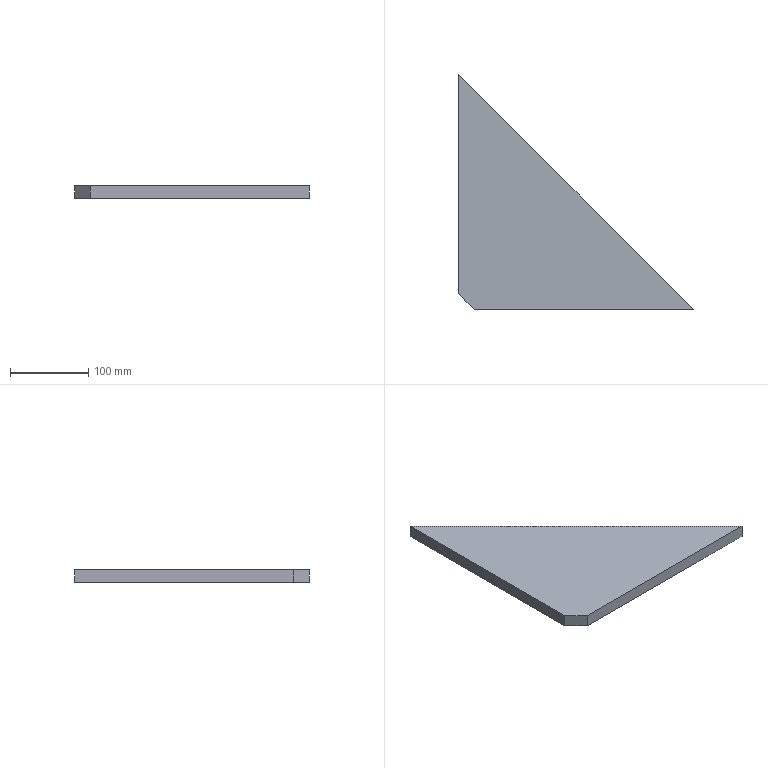Part | SolidWorks | features Chamfer 1, Extrusion 1 | 1 solid | 6 faces | box 300 x 300 x 16 mm | volume 716800 mm3 | plane 6
STEP:
#1=CARTESIAN_POINT('',(0.,20.,-8.));
#2=VERTEX_POINT('',#1);
#3=CARTESIAN_POINT('',(0.,300.,-8.));
#4=VERTEX_POINT('',#3);
#5=CARTESIAN_POINT('',(0.,0.,-8.));
#6=DIRECTION('',(0.,1.,0.));
#7=VECTOR('',#6,1000.);
#8=LINE('',#5,#7);
#9=EDGE_CURVE('',#2,#4,#8,.T.);
#10=ORIENTED_EDGE('',*,*,#9,.F.);
#11=CARTESIAN_POINT('',(0.,20.,8.));
#12=VERTEX_POINT('',#11);
#13=CARTESIAN_POINT('',(0.,20.,8.));
#14=DIRECTION('',(0.,0.,1.));
#15=VECTOR('',#14,1000.);
#16=LINE('',#13,#15);
#17=EDGE_CURVE('',#2,#12,#16,.T.);
#18=ORIENTED_EDGE('',*,*,#17,.T.);
#19=CARTESIAN_POINT('',(0.,300.,8.));
#20=VERTEX_POINT('',#19);
#21=CARTESIAN_POINT('',(0.,0.,8.));
#22=DIRECTION('',(0.,1.,0.));
#23=VECTOR('',#22,1000.);
#24=LINE('',#21,#23);
#25=EDGE_CURVE('',#12,#20,#24,.T.);
#26=ORIENTED_EDGE('',*,*,#25,.T.);
#27=CARTESIAN_POINT('',(0.,300.,8.));
#28=DIRECTION('',(0.,0.,-1.));
#29=VECTOR('',#28,1000.);
#30=LINE('',#27,#29);
#31=EDGE_CURVE('',#20,#4,#30,.T.);
#32=ORIENTED_EDGE('',*,*,#31,.T.);
#33=EDGE_LOOP('',(#10,#18,#26,#32));
#34=FACE_OUTER_BOUND('',#33,.T.);
#35=CARTESIAN_POINT('',(0.,0.,8.));
#36=DIRECTION('',(-1.,0.,0.));
#37=DIRECTION('',(0.,0.,1.));
#38=AXIS2_PLACEMENT_3D('',#35,#36,#37);
#39=PLANE('',#38);
#40=ADVANCED_FACE('',(#34),#39,.T.);
#41=CARTESIAN_POINT('',(300.,0.,8.));
#42=VERTEX_POINT('',#41);
#43=CARTESIAN_POINT('',(20.,0.,8.));
#44=VERTEX_POINT('',#43);
#45=CARTESIAN_POINT('',(300.,0.,8.));
#46=DIRECTION('',(-1.,0.,0.));
#47=VECTOR('',#46,1000.);
#48=LINE('',#45,#47);
#49=EDGE_CURVE('',#42,#44,#48,.T.);
#50=ORIENTED_EDGE('',*,*,#49,.T.);
#51=CARTESIAN_POINT('',(20.,0.,-8.));
#52=VERTEX_POINT('',#51);
#53=CARTESIAN_POINT('',(20.,0.,8.));
#54=DIRECTION('',(0.,0.,-1.));
#55=VECTOR('',#54,1000.);
#56=LINE('',#53,#55);
#57=EDGE_CURVE('',#44,#52,#56,.T.);
#58=ORIENTED_EDGE('',*,*,#57,.T.);
#59=CARTESIAN_POINT('',(300.,0.,-8.));
#60=VERTEX_POINT('',#59);
#61=CARTESIAN_POINT('',(300.,0.,-8.));
#62=DIRECTION('',(-1.,0.,0.));
#63=VECTOR('',#62,1000.);
#64=LINE('',#61,#63);
#65=EDGE_CURVE('',#60,#52,#64,.T.);
#66=ORIENTED_EDGE('',*,*,#65,.F.);
#67=CARTESIAN_POINT('',(300.,0.,8.));
#68=DIRECTION('',(0.,0.,-1.));
#69=VECTOR('',#68,1000.);
#70=LINE('',#67,#69);
#71=EDGE_CURVE('',#42,#60,#70,.T.);
#72=ORIENTED_EDGE('',*,*,#71,.F.);
#73=EDGE_LOOP('',(#50,#58,#66,#72));
#74=FACE_OUTER_BOUND('',#73,.T.);
#75=CARTESIAN_POINT('',(300.,0.,8.));
#76=DIRECTION('',(0.,-1.,0.));
#77=DIRECTION('',(0.,0.,-1.));
#78=AXIS2_PLACEMENT_3D('',#75,#76,#77);
#79=PLANE('',#78);
#80=ADVANCED_FACE('',(#74),#79,.T.);
#81=CARTESIAN_POINT('',(0.,300.,-8.));
#82=DIRECTION('',(0.7071,-0.7071,0.));
#83=VECTOR('',#82,1000.);
#84=LINE('',#81,#83);
#85=EDGE_CURVE('',#4,#60,#84,.T.);
#86=ORIENTED_EDGE('',*,*,#85,.F.);
#87=ORIENTED_EDGE('',*,*,#31,.F.);
#88=CARTESIAN_POINT('',(0.,300.,8.));
#89=DIRECTION('',(0.7071,-0.7071,0.));
#90=VECTOR('',#89,1000.);
#91=LINE('',#88,#90);
#92=EDGE_CURVE('',#20,#42,#91,.T.);
#93=ORIENTED_EDGE('',*,*,#92,.T.);
#94=ORIENTED_EDGE('',*,*,#71,.T.);
#95=EDGE_LOOP('',(#86,#87,#93,#94));
#96=FACE_OUTER_BOUND('',#95,.T.);
#97=CARTESIAN_POINT('',(0.,300.,8.));
#98=DIRECTION('',(0.7071,0.7071,0.));
#99=DIRECTION('',(-0.7071,0.7071,0.));
#100=AXIS2_PLACEMENT_3D('',#97,#98,#99);
#101=PLANE('',#100);
#102=ADVANCED_FACE('',(#96),#101,.T.);
#103=ORIENTED_EDGE('',*,*,#25,.F.);
#104=CARTESIAN_POINT('',(10.,10.,8.));
#105=DIRECTION('',(0.7071,-0.7071,0.));
#106=VECTOR('',#105,1000.);
#107=LINE('',#104,#106);
#108=EDGE_CURVE('',#12,#44,#107,.T.);
#109=ORIENTED_EDGE('',*,*,#108,.T.);
#110=ORIENTED_EDGE('',*,*,#49,.F.);
#111=ORIENTED_EDGE('',*,*,#92,.F.);
#112=EDGE_LOOP('',(#103,#109,#110,#111));
#113=FACE_OUTER_BOUND('',#112,.T.);
#114=CARTESIAN_POINT('',(0.,0.,8.));
#115=DIRECTION('',(0.,0.,1.));
#116=DIRECTION('',(1.,0.,0.));
#117=AXIS2_PLACEMENT_3D('',#114,#115,#116);
#118=PLANE('',#117);
#119=ADVANCED_FACE('',(#113),#118,.T.);
#120=ORIENTED_EDGE('',*,*,#65,.T.);
#121=CARTESIAN_POINT('',(20.,0.,-8.));
#122=DIRECTION('',(-0.7071,0.7071,0.));
#123=VECTOR('',#122,1000.);
#124=LINE('',#121,#123);
#125=EDGE_CURVE('',#52,#2,#124,.T.);
#126=ORIENTED_EDGE('',*,*,#125,.T.);
#127=ORIENTED_EDGE('',*,*,#9,.T.);
#128=ORIENTED_EDGE('',*,*,#85,.T.);
#129=EDGE_LOOP('',(#120,#126,#127,#128));
#130=FACE_OUTER_BOUND('',#129,.T.);
#131=CARTESIAN_POINT('',(0.,0.,-8.));
#132=DIRECTION('',(0.,0.,1.));
#133=DIRECTION('',(1.,0.,0.));
#134=AXIS2_PLACEMENT_3D('',#131,#132,#133);
#135=PLANE('',#134);
#136=ADVANCED_FACE('',(#130),#135,.F.);
#137=ORIENTED_EDGE('',*,*,#108,.F.);
#138=ORIENTED_EDGE('',*,*,#17,.F.);
#139=ORIENTED_EDGE('',*,*,#125,.F.);
#140=ORIENTED_EDGE('',*,*,#57,.F.);
#141=EDGE_LOOP('',(#137,#138,#139,#140));
#142=FACE_OUTER_BOUND('',#141,.T.);
#143=CARTESIAN_POINT('',(20.,0.,8.));
#144=DIRECTION('',(0.7071,0.7071,0.));
#145=DIRECTION('',(0.,0.,-1.));
#146=AXIS2_PLACEMENT_3D('',#143,#144,#145);
#147=PLANE('',#146);
#148=ADVANCED_FACE('',(#142),#147,.F.);
#149=CLOSED_SHELL('',(#40,#80,#102,#119,#136,#148));
#150=MANIFOLD_SOLID_BREP('',#149);
#151=CARTESIAN_POINT('',(0.,0.,0.));
#152=DIRECTION('',(0.,0.,1.));
#153=DIRECTION('',(1.,0.,0.));
#154=AXIS2_PLACEMENT_3D('',#151,#152,#153);
#155=(LENGTH_UNIT()NAMED_UNIT(*)SI_UNIT(.MILLI.,.METRE.));
#156=UNCERTAINTY_MEASURE_WITH_UNIT(LENGTH_MEASURE(0.00001),#155,'','');
#157=(NAMED_UNIT(*)PLANE_ANGLE_UNIT()SI_UNIT($,.RADIAN.));
#158=(NAMED_UNIT(*)SI_UNIT($,.STERADIAN.)SOLID_ANGLE_UNIT());
#159=(GEOMETRIC_REPRESENTATION_CONTEXT(3)GLOBAL_UNCERTAINTY_ASSIGNED_CONTEXT((#156))GLOBAL_UNIT_ASSIGNED_CONTEXT((#155,#157,#158))REPRESENTATION_CONTEXT('',''));
#160=ADVANCED_BREP_SHAPE_REPRESENTATION('',(#150,#154),#159);